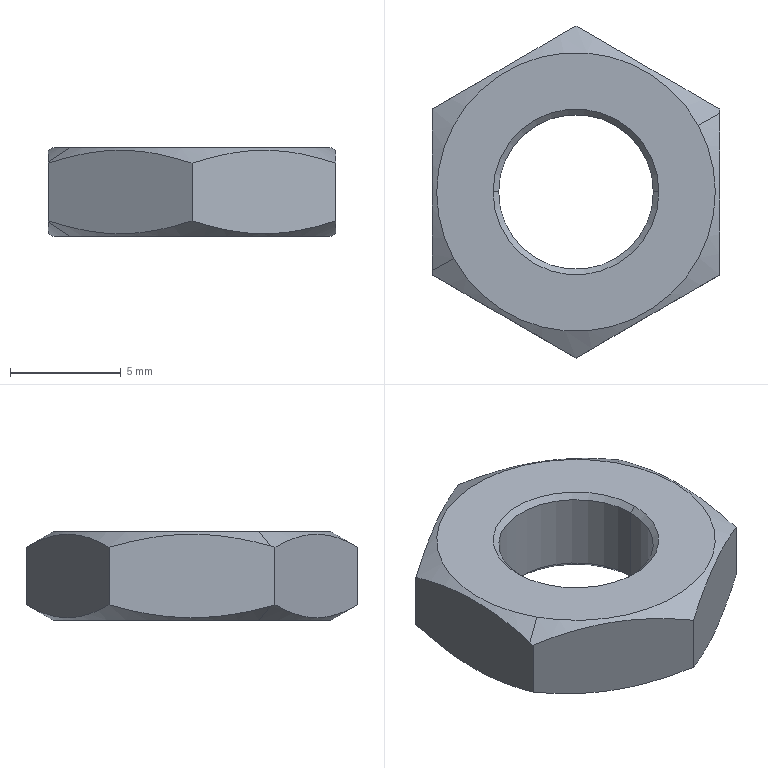Part | NX | features BREP 1 | 1 solid | 18 faces | box 13 x 15.011 x 4 mm | volume 421.241 mm3 | cone 8 | plane 8 | cylinder 2 | commonest cylinder face diameters 7 x2
STEP:
#1=CARTESIAN_POINT('',(3.75,0.,0.));
#2=VERTEX_POINT('',#1);
#3=CARTESIAN_POINT('',(3.5,0.,0.25));
#4=VERTEX_POINT('',#3);
#5=CARTESIAN_POINT('',(3.625,0.,0.125));
#6=DIRECTION('',(0.7071,0.,-0.7071));
#7=VECTOR('',#6,1000.);
#8=LINE('',#5,#7);
#9=EDGE_CURVE('',#2,#4,#8,.F.);
#10=ORIENTED_EDGE('',*,*,#9,.T.);
#11=CARTESIAN_POINT('',(-3.5,0.,0.25));
#12=VERTEX_POINT('',#11);
#13=CARTESIAN_POINT('',(0.,0.,0.25));
#14=DIRECTION('',(0.,0.,1.));
#15=DIRECTION('',(1.,0.,0.));
#16=AXIS2_PLACEMENT_3D('',#13,#14,#15);
#17=CIRCLE('',#16,3.5);
#18=EDGE_CURVE('',#4,#12,#17,.T.);
#19=ORIENTED_EDGE('',*,*,#18,.T.);
#20=CARTESIAN_POINT('',(-3.75,0.000000268,0.));
#21=VERTEX_POINT('',#20);
#22=CARTESIAN_POINT('',(-3.625,0.,0.125));
#23=DIRECTION('',(-0.7071,0.,-0.7071));
#24=VECTOR('',#23,1000.);
#25=LINE('',#22,#24);
#26=EDGE_CURVE('',#21,#12,#25,.F.);
#27=ORIENTED_EDGE('',*,*,#26,.F.);
#28=CARTESIAN_POINT('',(0.,0.,0.));
#29=DIRECTION('',(0.,0.,1.));
#30=DIRECTION('',(1.,0.,0.));
#31=AXIS2_PLACEMENT_3D('',#28,#29,#30);
#32=CIRCLE('',#31,3.75);
#33=EDGE_CURVE('',#2,#21,#32,.T.);
#34=ORIENTED_EDGE('',*,*,#33,.F.);
#35=EDGE_LOOP('',(#10,#19,#27,#34));
#36=FACE_BOUND('',#35,.T.);
#37=CARTESIAN_POINT('',(0.,0.,3.75));
#38=DIRECTION('',(0.,0.,-1.));
#39=DIRECTION('',(1.,0.,0.));
#40=AXIS2_PLACEMENT_3D('',#37,#38,#39);
#41=CONICAL_SURFACE('',#40,0.,0.7854);
#42=ADVANCED_FACE('',(#36),#41,.F.);
#43=ORIENTED_EDGE('',*,*,#26,.T.);
#44=CARTESIAN_POINT('',(0.,0.,0.25));
#45=DIRECTION('',(0.,0.,1.));
#46=DIRECTION('',(1.,0.,0.));
#47=AXIS2_PLACEMENT_3D('',#44,#45,#46);
#48=CIRCLE('',#47,3.5);
#49=EDGE_CURVE('',#12,#4,#48,.T.);
#50=ORIENTED_EDGE('',*,*,#49,.T.);
#51=ORIENTED_EDGE('',*,*,#9,.F.);
#52=CARTESIAN_POINT('',(0.,0.,0.));
#53=DIRECTION('',(0.,0.,1.));
#54=DIRECTION('',(1.,0.,0.));
#55=AXIS2_PLACEMENT_3D('',#52,#53,#54);
#56=CIRCLE('',#55,3.75);
#57=EDGE_CURVE('',#21,#2,#56,.T.);
#58=ORIENTED_EDGE('',*,*,#57,.F.);
#59=EDGE_LOOP('',(#43,#50,#51,#58));
#60=FACE_BOUND('',#59,.T.);
#61=CARTESIAN_POINT('',(0.,0.,3.75));
#62=DIRECTION('',(0.,0.,-1.));
#63=DIRECTION('',(-0.9924,0.1227,0.));
#64=AXIS2_PLACEMENT_3D('',#61,#62,#63);
#65=CONICAL_SURFACE('',#64,0.,0.7854);
#66=ADVANCED_FACE('',(#60),#65,.F.);
#67=ORIENTED_EDGE('',*,*,#49,.F.);
#68=CARTESIAN_POINT('',(-3.5,0.,3.75));
#69=VERTEX_POINT('',#68);
#70=CARTESIAN_POINT('',(-3.5,0.,2.));
#71=DIRECTION('',(0.,0.,1.));
#72=VECTOR('',#71,1000.);
#73=LINE('',#70,#72);
#74=EDGE_CURVE('',#12,#69,#73,.T.);
#75=ORIENTED_EDGE('',*,*,#74,.T.);
#76=CARTESIAN_POINT('',(3.5,0.,3.75));
#77=VERTEX_POINT('',#76);
#78=CARTESIAN_POINT('',(0.,0.,3.75));
#79=DIRECTION('',(0.,0.,1.));
#80=DIRECTION('',(1.,0.,0.));
#81=AXIS2_PLACEMENT_3D('',#78,#79,#80);
#82=CIRCLE('',#81,3.5);
#83=EDGE_CURVE('',#69,#77,#82,.T.);
#84=ORIENTED_EDGE('',*,*,#83,.T.);
#85=CARTESIAN_POINT('',(3.5,0.,2.));
#86=DIRECTION('',(0.,0.,1.));
#87=VECTOR('',#86,1000.);
#88=LINE('',#85,#87);
#89=EDGE_CURVE('',#4,#77,#88,.T.);
#90=ORIENTED_EDGE('',*,*,#89,.F.);
#91=EDGE_LOOP('',(#67,#75,#84,#90));
#92=FACE_BOUND('',#91,.T.);
#93=CARTESIAN_POINT('',(0.,0.,2.));
#94=DIRECTION('',(0.,0.,1.));
#95=DIRECTION('',(1.,0.,0.));
#96=AXIS2_PLACEMENT_3D('',#93,#94,#95);
#97=CYLINDRICAL_SURFACE('',#96,3.5);
#98=ADVANCED_FACE('',(#92),#97,.F.);
#99=ORIENTED_EDGE('',*,*,#18,.F.);
#100=ORIENTED_EDGE('',*,*,#89,.T.);
#101=CARTESIAN_POINT('',(0.,0.,3.75));
#102=DIRECTION('',(0.,0.,1.));
#103=DIRECTION('',(1.,0.,0.));
#104=AXIS2_PLACEMENT_3D('',#101,#102,#103);
#105=CIRCLE('',#104,3.5);
#106=EDGE_CURVE('',#77,#69,#105,.T.);
#107=ORIENTED_EDGE('',*,*,#106,.T.);
#108=ORIENTED_EDGE('',*,*,#74,.F.);
#109=EDGE_LOOP('',(#99,#100,#107,#108));
#110=FACE_BOUND('',#109,.T.);
#111=CARTESIAN_POINT('',(0.,0.,2.));
#112=DIRECTION('',(0.,0.,1.));
#113=DIRECTION('',(1.,0.,0.));
#114=AXIS2_PLACEMENT_3D('',#111,#112,#113);
#115=CYLINDRICAL_SURFACE('',#114,3.5);
#116=ADVANCED_FACE('',(#110),#115,.F.);
#117=ORIENTED_EDGE('',*,*,#57,.T.);
#118=ORIENTED_EDGE('',*,*,#33,.T.);
#119=EDGE_LOOP('',(#117,#118));
#120=FACE_BOUND('',#119,.T.);
#121=CARTESIAN_POINT('',(-5.529,-3.02,0.));
#122=VERTEX_POINT('',#121);
#123=CARTESIAN_POINT('',(5.529,3.02,0.));
#124=VERTEX_POINT('',#123);
#125=CARTESIAN_POINT('',(0.,0.,0.));
#126=DIRECTION('',(0.,0.,1.));
#127=DIRECTION('',(1.,0.,0.));
#128=AXIS2_PLACEMENT_3D('',#125,#126,#127);
#129=CIRCLE('',#128,6.3);
#130=EDGE_CURVE('',#122,#124,#129,.T.);
#131=ORIENTED_EDGE('',*,*,#130,.F.);
#132=CARTESIAN_POINT('',(0.,0.,0.));
#133=DIRECTION('',(0.,0.,1.));
#134=DIRECTION('',(1.,0.,0.));
#135=AXIS2_PLACEMENT_3D('',#132,#133,#134);
#136=CIRCLE('',#135,6.3);
#137=EDGE_CURVE('',#124,#122,#136,.T.);
#138=ORIENTED_EDGE('',*,*,#137,.F.);
#139=EDGE_LOOP('',(#131,#138));
#140=FACE_BOUND('',#139,.T.);
#141=CARTESIAN_POINT('',(0.,0.,0.));
#142=DIRECTION('',(0.,0.,1.));
#143=DIRECTION('',(1.,0.,0.));
#144=AXIS2_PLACEMENT_3D('',#141,#142,#143);
#145=PLANE('',#144);
#146=ADVANCED_FACE('',(#120,#140),#145,.F.);
#147=CARTESIAN_POINT('',(3.75,0.,4.));
#148=VERTEX_POINT('',#147);
#149=CARTESIAN_POINT('',(3.625,0.,3.875));
#150=DIRECTION('',(0.7071,0.,0.7071));
#151=VECTOR('',#150,1000.);
#152=LINE('',#149,#151);
#153=EDGE_CURVE('',#148,#77,#152,.F.);
#154=ORIENTED_EDGE('',*,*,#153,.F.);
#155=CARTESIAN_POINT('',(-3.75,0.000000268,4.));
#156=VERTEX_POINT('',#155);
#157=CARTESIAN_POINT('',(0.,0.,4.));
#158=DIRECTION('',(0.,0.,1.));
#159=DIRECTION('',(1.,0.,0.));
#160=AXIS2_PLACEMENT_3D('',#157,#158,#159);
#161=CIRCLE('',#160,3.75);
#162=EDGE_CURVE('',#148,#156,#161,.T.);
#163=ORIENTED_EDGE('',*,*,#162,.T.);
#164=CARTESIAN_POINT('',(-3.625,0.000000218,3.875));
#165=DIRECTION('',(-0.7071,0.000000043,0.7071));
#166=VECTOR('',#165,1000.);
#167=LINE('',#164,#166);
#168=EDGE_CURVE('',#156,#69,#167,.F.);
#169=ORIENTED_EDGE('',*,*,#168,.T.);
#170=ORIENTED_EDGE('',*,*,#106,.F.);
#171=EDGE_LOOP('',(#154,#163,#169,#170));
#172=FACE_BOUND('',#171,.T.);
#173=CARTESIAN_POINT('',(0.,0.,0.25));
#174=DIRECTION('',(0.,0.,1.));
#175=DIRECTION('',(1.,0.,0.));
#176=AXIS2_PLACEMENT_3D('',#173,#174,#175);
#177=CONICAL_SURFACE('',#176,0.,0.7854);
#178=ADVANCED_FACE('',(#172),#177,.F.);
#179=ORIENTED_EDGE('',*,*,#168,.F.);
#180=CARTESIAN_POINT('',(0.,0.,4.));
#181=DIRECTION('',(0.,0.,1.));
#182=DIRECTION('',(1.,0.,0.));
#183=AXIS2_PLACEMENT_3D('',#180,#181,#182);
#184=CIRCLE('',#183,3.75);
#185=EDGE_CURVE('',#156,#148,#184,.T.);
#186=ORIENTED_EDGE('',*,*,#185,.T.);
#187=ORIENTED_EDGE('',*,*,#153,.T.);
#188=ORIENTED_EDGE('',*,*,#83,.F.);
#189=EDGE_LOOP('',(#179,#186,#187,#188));
#190=FACE_BOUND('',#189,.T.);
#191=CARTESIAN_POINT('',(0.,0.,0.25));
#192=DIRECTION('',(0.,0.,1.));
#193=DIRECTION('',(-0.9924,0.1227,0.));
#194=AXIS2_PLACEMENT_3D('',#191,#192,#193);
#195=CONICAL_SURFACE('',#194,0.,0.7854);
#196=ADVANCED_FACE('',(#190),#195,.F.);
#197=ORIENTED_EDGE('',*,*,#162,.F.);
#198=ORIENTED_EDGE('',*,*,#185,.F.);
#199=EDGE_LOOP('',(#197,#198));
#200=FACE_BOUND('',#199,.T.);
#201=CARTESIAN_POINT('',(-5.529,-3.02,4.));
#202=VERTEX_POINT('',#201);
#203=CARTESIAN_POINT('',(5.529,3.02,4.));
#204=VERTEX_POINT('',#203);
#205=CARTESIAN_POINT('',(0.,0.,4.));
#206=DIRECTION('',(0.,0.,-1.));
#207=DIRECTION('',(-1.,0.,0.));
#208=AXIS2_PLACEMENT_3D('',#205,#206,#207);
#209=CIRCLE('',#208,6.3);
#210=EDGE_CURVE('',#202,#204,#209,.T.);
#211=ORIENTED_EDGE('',*,*,#210,.F.);
#212=CARTESIAN_POINT('',(0.,0.,4.));
#213=DIRECTION('',(0.,0.,-1.));
#214=DIRECTION('',(-1.,0.,0.));
#215=AXIS2_PLACEMENT_3D('',#212,#213,#214);
#216=CIRCLE('',#215,6.3);
#217=EDGE_CURVE('',#204,#202,#216,.T.);
#218=ORIENTED_EDGE('',*,*,#217,.F.);
#219=EDGE_LOOP('',(#211,#218));
#220=FACE_BOUND('',#219,.T.);
#221=CARTESIAN_POINT('',(0.,0.,4.));
#222=DIRECTION('',(0.,0.,1.));
#223=DIRECTION('',(1.,0.,0.));
#224=AXIS2_PLACEMENT_3D('',#221,#222,#223);
#225=PLANE('',#224);
#226=ADVANCED_FACE('',(#200,#220),#225,.T.);
#227=CARTESIAN_POINT('',(-6.5,-3.551,0.639));
#228=VERTEX_POINT('',#227);
#229=CARTESIAN_POINT('',(-6.788,-3.708,0.8285));
#230=DIRECTION('',(-0.76,-0.4152,0.5));
#231=VECTOR('',#230,1000.);
#232=LINE('',#229,#231);
#233=EDGE_CURVE('',#122,#228,#232,.T.);
#234=ORIENTED_EDGE('',*,*,#233,.F.);
#235=ORIENTED_EDGE('',*,*,#130,.T.);
#236=CARTESIAN_POINT('',(6.5,3.551,0.639));
#237=VERTEX_POINT('',#236);
#238=CARTESIAN_POINT('',(6.788,3.708,0.8285));
#239=DIRECTION('',(0.76,0.4152,0.5));
#240=VECTOR('',#239,1000.);
#241=LINE('',#238,#240);
#242=EDGE_CURVE('',#124,#237,#241,.T.);
#243=ORIENTED_EDGE('',*,*,#242,.T.);
#244=CARTESIAN_POINT('',(6.5,-3.753,0.696));
#245=VERTEX_POINT('',#244);
#246=CARTESIAN_POINT('',(6.5,3.551,0.639));
#247=CARTESIAN_POINT('',(6.5,3.11,0.517));
#248=CARTESIAN_POINT('',(6.5,2.701,0.4182));
#249=CARTESIAN_POINT('',(6.5,2.313,0.338));
#250=CARTESIAN_POINT('',(6.5,1.299,0.1635));
#251=CARTESIAN_POINT('',(6.5,0.3692,0.09904));
#252=CARTESIAN_POINT('',(6.5,-0.2087,0.09497));
#253=CARTESIAN_POINT('',(6.5,-1.197,0.1497));
#254=CARTESIAN_POINT('',(6.5,-2.27,0.3265));
#255=CARTESIAN_POINT('',(6.5,-2.727,0.4207));
#256=CARTESIAN_POINT('',(6.5,-3.216,0.5412));
#257=CARTESIAN_POINT('',(6.5,-3.753,0.696));
#258=B_SPLINE_CURVE_WITH_KNOTS('',5,(#246,#247,#248,#249,#250,#251,#252,#253,#254,#255,#256,#257),.UNSPECIFIED.,.F.,.F.,(6,3,3,6),(0.,26.231,71.597,102.705),.UNSPECIFIED.);
#259=EDGE_CURVE('',#237,#245,#258,.T.);
#260=ORIENTED_EDGE('',*,*,#259,.T.);
#261=CARTESIAN_POINT('',(0.,-7.506,0.696));
#262=VERTEX_POINT('',#261);
#263=CARTESIAN_POINT('',(0.,-7.506,0.696));
#264=CARTESIAN_POINT('',(0.3698,-7.292,0.5728));
#265=CARTESIAN_POINT('',(0.7137,-7.094,0.4713));
#266=CARTESIAN_POINT('',(1.039,-6.906,0.3874));
#267=CARTESIAN_POINT('',(2.057,-6.318,0.1629));
#268=CARTESIAN_POINT('',(2.963,-5.795,0.08633));
#269=CARTESIAN_POINT('',(3.578,-5.44,0.08782));
#270=CARTESIAN_POINT('',(4.478,-4.92,0.1681));
#271=CARTESIAN_POINT('',(5.491,-4.335,0.3951));
#272=CARTESIAN_POINT('',(5.807,-4.153,0.4774));
#273=CARTESIAN_POINT('',(6.141,-3.96,0.5765));
#274=CARTESIAN_POINT('',(6.5,-3.753,0.696));
#275=B_SPLINE_CURVE_WITH_KNOTS('',5,(#263,#264,#265,#266,#267,#268,#269,#270,#271,#272,#273,#274),.UNSPECIFIED.,.F.,.F.,(6,3,3,6),(0.,24.765,81.109,105.126),.UNSPECIFIED.);
#276=EDGE_CURVE('',#262,#245,#275,.T.);
#277=ORIENTED_EDGE('',*,*,#276,.F.);
#278=CARTESIAN_POINT('',(-6.5,-3.753,0.696));
#279=VERTEX_POINT('',#278);
#280=CARTESIAN_POINT('',(-6.5,-3.753,0.696));
#281=CARTESIAN_POINT('',(-6.13,-3.966,0.5728));
#282=CARTESIAN_POINT('',(-5.786,-4.165,0.4713));
#283=CARTESIAN_POINT('',(-5.461,-4.352,0.3874));
#284=CARTESIAN_POINT('',(-4.443,-4.94,0.1629));
#285=CARTESIAN_POINT('',(-3.537,-5.464,0.08633));
#286=CARTESIAN_POINT('',(-2.922,-5.819,0.08782));
#287=CARTESIAN_POINT('',(-2.022,-6.338,0.1681));
#288=CARTESIAN_POINT('',(-1.009,-6.923,0.3951));
#289=CARTESIAN_POINT('',(-0.6929,-7.106,0.4774));
#290=CARTESIAN_POINT('',(-0.3586,-7.299,0.5765));
#291=CARTESIAN_POINT('',(0.,-7.506,0.696));
#292=B_SPLINE_CURVE_WITH_KNOTS('',5,(#280,#281,#282,#283,#284,#285,#286,#287,#288,#289,#290,#291),.UNSPECIFIED.,.F.,.F.,(6,3,3,6),(0.,24.765,81.109,105.126),.UNSPECIFIED.);
#293=EDGE_CURVE('',#279,#262,#292,.T.);
#294=ORIENTED_EDGE('',*,*,#293,.F.);
#295=CARTESIAN_POINT('',(-6.5,-3.551,0.639));
#296=CARTESIAN_POINT('',(-6.5,-3.591,0.65));
#297=CARTESIAN_POINT('',(-6.5,-3.631,0.6612));
#298=CARTESIAN_POINT('',(-6.5,-3.671,0.6726));
#299=CARTESIAN_POINT('',(-6.5,-3.712,0.6842));
#300=CARTESIAN_POINT('',(-6.5,-3.753,0.696));
#301=B_SPLINE_CURVE_WITH_KNOTS('',5,(#295,#296,#297,#298,#299,#300),.UNSPECIFIED.,.F.,.F.,(6,6),(0.,2.372),.UNSPECIFIED.);
#302=EDGE_CURVE('',#228,#279,#301,.T.);
#303=ORIENTED_EDGE('',*,*,#302,.F.);
#304=EDGE_LOOP('',(#234,#235,#243,#260,#277,#294,#303));
#305=FACE_BOUND('',#304,.T.);
#306=CARTESIAN_POINT('',(0.,0.,0.));
#307=DIRECTION('',(0.,0.,1.));
#308=DIRECTION('',(-0.8776,-0.4794,0.));
#309=AXIS2_PLACEMENT_3D('',#306,#307,#308);
#310=CONICAL_SURFACE('',#309,6.3,1.047);
#311=ADVANCED_FACE('',(#305),#310,.T.);
#312=ORIENTED_EDGE('',*,*,#242,.F.);
#313=ORIENTED_EDGE('',*,*,#137,.T.);
#314=ORIENTED_EDGE('',*,*,#233,.T.);
#315=CARTESIAN_POINT('',(-6.5,3.753,0.696));
#316=VERTEX_POINT('',#315);
#317=CARTESIAN_POINT('',(-6.5,-3.551,0.639));
#318=CARTESIAN_POINT('',(-6.5,-3.11,0.517));
#319=CARTESIAN_POINT('',(-6.5,-2.701,0.4182));
#320=CARTESIAN_POINT('',(-6.5,-2.313,0.338));
#321=CARTESIAN_POINT('',(-6.5,-1.299,0.1635));
#322=CARTESIAN_POINT('',(-6.5,-0.3692,0.09904));
#323=CARTESIAN_POINT('',(-6.5,0.2087,0.09497));
#324=CARTESIAN_POINT('',(-6.5,1.197,0.1497));
#325=CARTESIAN_POINT('',(-6.5,2.27,0.3265));
#326=CARTESIAN_POINT('',(-6.5,2.727,0.4207));
#327=CARTESIAN_POINT('',(-6.5,3.216,0.5412));
#328=CARTESIAN_POINT('',(-6.5,3.753,0.696));
#329=B_SPLINE_CURVE_WITH_KNOTS('',5,(#317,#318,#319,#320,#321,#322,#323,#324,#325,#326,#327,#328),.UNSPECIFIED.,.F.,.F.,(6,3,3,6),(0.,26.231,71.597,102.705),.UNSPECIFIED.);
#330=EDGE_CURVE('',#228,#316,#329,.T.);
#331=ORIENTED_EDGE('',*,*,#330,.T.);
#332=CARTESIAN_POINT('',(0.,7.506,0.696));
#333=VERTEX_POINT('',#332);
#334=CARTESIAN_POINT('',(0.,7.506,0.696));
#335=CARTESIAN_POINT('',(-0.3698,7.292,0.5728));
#336=CARTESIAN_POINT('',(-0.7137,7.094,0.4713));
#337=CARTESIAN_POINT('',(-1.039,6.906,0.3874));
#338=CARTESIAN_POINT('',(-2.057,6.318,0.1629));
#339=CARTESIAN_POINT('',(-2.963,5.795,0.08633));
#340=CARTESIAN_POINT('',(-3.578,5.44,0.08782));
#341=CARTESIAN_POINT('',(-4.478,4.92,0.1681));
#342=CARTESIAN_POINT('',(-5.491,4.335,0.3951));
#343=CARTESIAN_POINT('',(-5.807,4.153,0.4774));
#344=CARTESIAN_POINT('',(-6.141,3.96,0.5765));
#345=CARTESIAN_POINT('',(-6.5,3.753,0.696));
#346=B_SPLINE_CURVE_WITH_KNOTS('',5,(#334,#335,#336,#337,#338,#339,#340,#341,#342,#343,#344,#345),.UNSPECIFIED.,.F.,.F.,(6,3,3,6),(0.,24.765,81.109,105.126),.UNSPECIFIED.);
#347=EDGE_CURVE('',#333,#316,#346,.T.);
#348=ORIENTED_EDGE('',*,*,#347,.F.);
#349=CARTESIAN_POINT('',(6.5,3.753,0.696));
#350=VERTEX_POINT('',#349);
#351=CARTESIAN_POINT('',(6.5,3.753,0.696));
#352=CARTESIAN_POINT('',(6.13,3.966,0.5728));
#353=CARTESIAN_POINT('',(5.786,4.165,0.4713));
#354=CARTESIAN_POINT('',(5.461,4.352,0.3874));
#355=CARTESIAN_POINT('',(4.443,4.94,0.1629));
#356=CARTESIAN_POINT('',(3.537,5.464,0.08633));
#357=CARTESIAN_POINT('',(2.922,5.819,0.08782));
#358=CARTESIAN_POINT('',(2.022,6.338,0.1681));
#359=CARTESIAN_POINT('',(1.009,6.923,0.3951));
#360=CARTESIAN_POINT('',(0.6929,7.106,0.4774));
#361=CARTESIAN_POINT('',(0.3586,7.299,0.5765));
#362=CARTESIAN_POINT('',(0.,7.506,0.696));
#363=B_SPLINE_CURVE_WITH_KNOTS('',5,(#351,#352,#353,#354,#355,#356,#357,#358,#359,#360,#361,#362),.UNSPECIFIED.,.F.,.F.,(6,3,3,6),(0.,24.765,81.109,105.126),.UNSPECIFIED.);
#364=EDGE_CURVE('',#350,#333,#363,.T.);
#365=ORIENTED_EDGE('',*,*,#364,.F.);
#366=CARTESIAN_POINT('',(6.5,3.551,0.639));
#367=CARTESIAN_POINT('',(6.5,3.591,0.65));
#368=CARTESIAN_POINT('',(6.5,3.631,0.6612));
#369=CARTESIAN_POINT('',(6.5,3.671,0.6726));
#370=CARTESIAN_POINT('',(6.5,3.712,0.6842));
#371=CARTESIAN_POINT('',(6.5,3.753,0.696));
#372=B_SPLINE_CURVE_WITH_KNOTS('',5,(#366,#367,#368,#369,#370,#371),.UNSPECIFIED.,.F.,.F.,(6,6),(0.,2.372),.UNSPECIFIED.);
#373=EDGE_CURVE('',#237,#350,#372,.T.);
#374=ORIENTED_EDGE('',*,*,#373,.F.);
#375=EDGE_LOOP('',(#312,#313,#314,#331,#348,#365,#374));
#376=FACE_BOUND('',#375,.T.);
#377=CARTESIAN_POINT('',(0.,0.,0.));
#378=DIRECTION('',(0.,0.,1.));
#379=DIRECTION('',(-0.8776,-0.4794,0.));
#380=AXIS2_PLACEMENT_3D('',#377,#378,#379);
#381=CONICAL_SURFACE('',#380,6.3,1.047);
#382=ADVANCED_FACE('',(#376),#381,.T.);
#383=CARTESIAN_POINT('',(6.5,-3.753,3.304));
#384=VERTEX_POINT('',#383);
#385=CARTESIAN_POINT('',(6.5,-3.753,2.));
#386=DIRECTION('',(0.,0.,1.));
#387=VECTOR('',#386,1000.);
#388=LINE('',#385,#387);
#389=EDGE_CURVE('',#245,#384,#388,.T.);
#390=ORIENTED_EDGE('',*,*,#389,.T.);
#391=CARTESIAN_POINT('',(0.,-7.506,3.304));
#392=VERTEX_POINT('',#391);
#393=CARTESIAN_POINT('',(0.,-7.506,3.304));
#394=CARTESIAN_POINT('',(0.4257,-7.26,3.446));
#395=CARTESIAN_POINT('',(0.8172,-7.034,3.559));
#396=CARTESIAN_POINT('',(1.185,-6.822,3.649));
#397=CARTESIAN_POINT('',(2.094,-6.297,3.834));
#398=CARTESIAN_POINT('',(2.925,-5.817,3.901));
#399=CARTESIAN_POINT('',(3.425,-5.528,3.905));
#400=CARTESIAN_POINT('',(4.282,-5.033,3.851));
#401=CARTESIAN_POINT('',(5.212,-4.497,3.674));
#402=CARTESIAN_POINT('',(5.609,-4.267,3.58));
#403=CARTESIAN_POINT('',(6.034,-4.022,3.459));
#404=CARTESIAN_POINT('',(6.5,-3.753,3.304));
#405=B_SPLINE_CURVE_WITH_KNOTS('',5,(#393,#394,#395,#396,#397,#398,#399,#400,#401,#402,#403,#404),.UNSPECIFIED.,.F.,.F.,(6,3,3,6),(0.,28.513,73.873,105.079),.UNSPECIFIED.);
#406=EDGE_CURVE('',#392,#384,#405,.T.);
#407=ORIENTED_EDGE('',*,*,#406,.F.);
#408=CARTESIAN_POINT('',(0.,-7.506,2.));
#409=DIRECTION('',(0.,0.,1.));
#410=VECTOR('',#409,1000.);
#411=LINE('',#408,#410);
#412=EDGE_CURVE('',#262,#392,#411,.T.);
#413=ORIENTED_EDGE('',*,*,#412,.F.);
#414=ORIENTED_EDGE('',*,*,#276,.T.);
#415=EDGE_LOOP('',(#390,#407,#413,#414));
#416=FACE_BOUND('',#415,.T.);
#417=CARTESIAN_POINT('',(0.,-7.506,0.));
#418=DIRECTION('',(0.5,-0.866,0.));
#419=DIRECTION('',(0.866,0.5,0.));
#420=AXIS2_PLACEMENT_3D('',#417,#418,#419);
#421=PLANE('',#420);
#422=ADVANCED_FACE('',(#416),#421,.T.);
#423=ORIENTED_EDGE('',*,*,#412,.T.);
#424=CARTESIAN_POINT('',(-6.5,-3.753,3.304));
#425=VERTEX_POINT('',#424);
#426=CARTESIAN_POINT('',(-6.5,-3.753,3.304));
#427=CARTESIAN_POINT('',(-6.074,-3.999,3.446));
#428=CARTESIAN_POINT('',(-5.683,-4.225,3.559));
#429=CARTESIAN_POINT('',(-5.315,-4.437,3.649));
#430=CARTESIAN_POINT('',(-4.406,-4.962,3.834));
#431=CARTESIAN_POINT('',(-3.575,-5.441,3.901));
#432=CARTESIAN_POINT('',(-3.075,-5.73,3.905));
#433=CARTESIAN_POINT('',(-2.218,-6.225,3.851));
#434=CARTESIAN_POINT('',(-1.288,-6.762,3.674));
#435=CARTESIAN_POINT('',(-0.8908,-6.991,3.58));
#436=CARTESIAN_POINT('',(-0.466,-7.237,3.459));
#437=CARTESIAN_POINT('',(0.,-7.506,3.304));
#438=B_SPLINE_CURVE_WITH_KNOTS('',5,(#426,#427,#428,#429,#430,#431,#432,#433,#434,#435,#436,#437),.UNSPECIFIED.,.F.,.F.,(6,3,3,6),(0.,28.513,73.873,105.079),.UNSPECIFIED.);
#439=EDGE_CURVE('',#425,#392,#438,.T.);
#440=ORIENTED_EDGE('',*,*,#439,.F.);
#441=CARTESIAN_POINT('',(-6.5,-3.753,2.));
#442=DIRECTION('',(0.,0.,1.));
#443=VECTOR('',#442,1000.);
#444=LINE('',#441,#443);
#445=EDGE_CURVE('',#279,#425,#444,.T.);
#446=ORIENTED_EDGE('',*,*,#445,.F.);
#447=ORIENTED_EDGE('',*,*,#293,.T.);
#448=EDGE_LOOP('',(#423,#440,#446,#447));
#449=FACE_BOUND('',#448,.T.);
#450=CARTESIAN_POINT('',(-6.5,-3.753,0.));
#451=DIRECTION('',(-0.5,-0.866,0.));
#452=DIRECTION('',(0.866,-0.5,0.));
#453=AXIS2_PLACEMENT_3D('',#450,#451,#452);
#454=PLANE('',#453);
#455=ADVANCED_FACE('',(#449),#454,.T.);
#456=ORIENTED_EDGE('',*,*,#445,.T.);
#457=CARTESIAN_POINT('',(-6.5,-3.551,3.361));
#458=VERTEX_POINT('',#457);
#459=CARTESIAN_POINT('',(-6.5,-3.551,3.361));
#460=CARTESIAN_POINT('',(-6.5,-3.617,3.343));
#461=CARTESIAN_POINT('',(-6.5,-3.685,3.324));
#462=CARTESIAN_POINT('',(-6.5,-3.753,3.304));
#463=B_SPLINE_CURVE_WITH_KNOTS('',3,(#459,#460,#461,#462),.UNSPECIFIED.,.F.,.F.,(4,4),(0.,2.372),.UNSPECIFIED.);
#464=EDGE_CURVE('',#458,#425,#463,.T.);
#465=ORIENTED_EDGE('',*,*,#464,.F.);
#466=CARTESIAN_POINT('',(-6.5,3.753,3.304));
#467=VERTEX_POINT('',#466);
#468=CARTESIAN_POINT('',(-6.5,-3.551,3.361));
#469=CARTESIAN_POINT('',(-6.5,-2.869,3.55));
#470=CARTESIAN_POINT('',(-6.5,-1.568,3.822));
#471=CARTESIAN_POINT('',(-6.5,0.07587,3.92));
#472=CARTESIAN_POINT('',(-6.5,1.727,3.8));
#473=CARTESIAN_POINT('',(-6.5,3.055,3.505));
#474=CARTESIAN_POINT('',(-6.5,3.753,3.304));
#475=B_SPLINE_CURVE_WITH_KNOTS('',3,(#468,#469,#470,#471,#472,#473,#474),.UNSPECIFIED.,.F.,.F.,(4,1,1,1,4),(0.,0.25,0.5,0.75,1.),.UNSPECIFIED.);
#476=EDGE_CURVE('',#458,#467,#475,.T.);
#477=ORIENTED_EDGE('',*,*,#476,.T.);
#478=CARTESIAN_POINT('',(-6.5,3.753,2.));
#479=DIRECTION('',(0.,0.,1.));
#480=VECTOR('',#479,1000.);
#481=LINE('',#478,#480);
#482=EDGE_CURVE('',#316,#467,#481,.T.);
#483=ORIENTED_EDGE('',*,*,#482,.F.);
#484=ORIENTED_EDGE('',*,*,#330,.F.);
#485=ORIENTED_EDGE('',*,*,#302,.T.);
#486=EDGE_LOOP('',(#456,#465,#477,#483,#484,#485));
#487=FACE_BOUND('',#486,.T.);
#488=CARTESIAN_POINT('',(-6.5,3.753,0.));
#489=DIRECTION('',(-1.,0.,0.));
#490=DIRECTION('',(0.,-1.,0.));
#491=AXIS2_PLACEMENT_3D('',#488,#489,#490);
#492=PLANE('',#491);
#493=ADVANCED_FACE('',(#487),#492,.T.);
#494=ORIENTED_EDGE('',*,*,#482,.T.);
#495=CARTESIAN_POINT('',(0.,7.506,3.304));
#496=VERTEX_POINT('',#495);
#497=CARTESIAN_POINT('',(0.,7.506,3.304));
#498=CARTESIAN_POINT('',(-0.4257,7.26,3.446));
#499=CARTESIAN_POINT('',(-0.8172,7.034,3.559));
#500=CARTESIAN_POINT('',(-1.185,6.822,3.649));
#501=CARTESIAN_POINT('',(-2.094,6.297,3.834));
#502=CARTESIAN_POINT('',(-2.925,5.817,3.901));
#503=CARTESIAN_POINT('',(-3.425,5.528,3.905));
#504=CARTESIAN_POINT('',(-4.282,5.033,3.851));
#505=CARTESIAN_POINT('',(-5.212,4.497,3.674));
#506=CARTESIAN_POINT('',(-5.609,4.267,3.58));
#507=CARTESIAN_POINT('',(-6.034,4.022,3.459));
#508=CARTESIAN_POINT('',(-6.5,3.753,3.304));
#509=B_SPLINE_CURVE_WITH_KNOTS('',5,(#497,#498,#499,#500,#501,#502,#503,#504,#505,#506,#507,#508),.UNSPECIFIED.,.F.,.F.,(6,3,3,6),(0.,28.513,73.873,105.079),.UNSPECIFIED.);
#510=EDGE_CURVE('',#496,#467,#509,.T.);
#511=ORIENTED_EDGE('',*,*,#510,.F.);
#512=CARTESIAN_POINT('',(0.,7.506,2.));
#513=DIRECTION('',(0.,0.,1.));
#514=VECTOR('',#513,1000.);
#515=LINE('',#512,#514);
#516=EDGE_CURVE('',#333,#496,#515,.T.);
#517=ORIENTED_EDGE('',*,*,#516,.F.);
#518=ORIENTED_EDGE('',*,*,#347,.T.);
#519=EDGE_LOOP('',(#494,#511,#517,#518));
#520=FACE_BOUND('',#519,.T.);
#521=CARTESIAN_POINT('',(0.,7.506,0.));
#522=DIRECTION('',(-0.5,0.866,0.));
#523=DIRECTION('',(-0.866,-0.5,0.));
#524=AXIS2_PLACEMENT_3D('',#521,#522,#523);
#525=PLANE('',#524);
#526=ADVANCED_FACE('',(#520),#525,.T.);
#527=ORIENTED_EDGE('',*,*,#516,.T.);
#528=CARTESIAN_POINT('',(6.5,3.753,3.304));
#529=VERTEX_POINT('',#528);
#530=CARTESIAN_POINT('',(6.5,3.753,3.304));
#531=CARTESIAN_POINT('',(6.074,3.999,3.446));
#532=CARTESIAN_POINT('',(5.683,4.225,3.559));
#533=CARTESIAN_POINT('',(5.315,4.437,3.649));
#534=CARTESIAN_POINT('',(4.406,4.962,3.834));
#535=CARTESIAN_POINT('',(3.575,5.441,3.901));
#536=CARTESIAN_POINT('',(3.075,5.73,3.905));
#537=CARTESIAN_POINT('',(2.218,6.225,3.851));
#538=CARTESIAN_POINT('',(1.288,6.762,3.674));
#539=CARTESIAN_POINT('',(0.8908,6.991,3.58));
#540=CARTESIAN_POINT('',(0.466,7.237,3.459));
#541=CARTESIAN_POINT('',(0.,7.506,3.304));
#542=B_SPLINE_CURVE_WITH_KNOTS('',5,(#530,#531,#532,#533,#534,#535,#536,#537,#538,#539,#540,#541),.UNSPECIFIED.,.F.,.F.,(6,3,3,6),(0.,28.513,73.873,105.079),.UNSPECIFIED.);
#543=EDGE_CURVE('',#529,#496,#542,.T.);
#544=ORIENTED_EDGE('',*,*,#543,.F.);
#545=CARTESIAN_POINT('',(6.5,3.753,2.));
#546=DIRECTION('',(0.,0.,1.));
#547=VECTOR('',#546,1000.);
#548=LINE('',#545,#547);
#549=EDGE_CURVE('',#350,#529,#548,.T.);
#550=ORIENTED_EDGE('',*,*,#549,.F.);
#551=ORIENTED_EDGE('',*,*,#364,.T.);
#552=EDGE_LOOP('',(#527,#544,#550,#551));
#553=FACE_BOUND('',#552,.T.);
#554=CARTESIAN_POINT('',(6.5,3.753,0.));
#555=DIRECTION('',(0.5,0.866,0.));
#556=DIRECTION('',(-0.866,0.5,0.));
#557=AXIS2_PLACEMENT_3D('',#554,#555,#556);
#558=PLANE('',#557);
#559=ADVANCED_FACE('',(#553),#558,.T.);
#560=ORIENTED_EDGE('',*,*,#549,.T.);
#561=CARTESIAN_POINT('',(6.5,3.551,3.361));
#562=VERTEX_POINT('',#561);
#563=CARTESIAN_POINT('',(6.5,3.551,3.361));
#564=CARTESIAN_POINT('',(6.5,3.617,3.343));
#565=CARTESIAN_POINT('',(6.5,3.685,3.324));
#566=CARTESIAN_POINT('',(6.5,3.753,3.304));
#567=B_SPLINE_CURVE_WITH_KNOTS('',3,(#563,#564,#565,#566),.UNSPECIFIED.,.F.,.F.,(4,4),(0.,2.372),.UNSPECIFIED.);
#568=EDGE_CURVE('',#562,#529,#567,.T.);
#569=ORIENTED_EDGE('',*,*,#568,.F.);
#570=CARTESIAN_POINT('',(6.5,3.551,3.361));
#571=CARTESIAN_POINT('',(6.5,2.869,3.55));
#572=CARTESIAN_POINT('',(6.5,1.568,3.822));
#573=CARTESIAN_POINT('',(6.5,-0.07587,3.92));
#574=CARTESIAN_POINT('',(6.5,-1.727,3.8));
#575=CARTESIAN_POINT('',(6.5,-3.055,3.505));
#576=CARTESIAN_POINT('',(6.5,-3.753,3.304));
#577=B_SPLINE_CURVE_WITH_KNOTS('',3,(#570,#571,#572,#573,#574,#575,#576),.UNSPECIFIED.,.F.,.F.,(4,1,1,1,4),(0.,0.25,0.5,0.75,1.),.UNSPECIFIED.);
#578=EDGE_CURVE('',#562,#384,#577,.T.);
#579=ORIENTED_EDGE('',*,*,#578,.T.);
#580=ORIENTED_EDGE('',*,*,#389,.F.);
#581=ORIENTED_EDGE('',*,*,#259,.F.);
#582=ORIENTED_EDGE('',*,*,#373,.T.);
#583=EDGE_LOOP('',(#560,#569,#579,#580,#581,#582));
#584=FACE_BOUND('',#583,.T.);
#585=CARTESIAN_POINT('',(6.5,-3.753,0.));
#586=DIRECTION('',(1.,0.,0.));
#587=DIRECTION('',(0.,1.,0.));
#588=AXIS2_PLACEMENT_3D('',#585,#586,#587);
#589=PLANE('',#588);
#590=ADVANCED_FACE('',(#584),#589,.T.);
#591=CARTESIAN_POINT('',(8.684,4.744,1.924));
#592=DIRECTION('',(0.76,0.4152,-0.5));
#593=VECTOR('',#592,1000.);
#594=LINE('',#591,#593);
#595=EDGE_CURVE('',#562,#204,#594,.F.);
#596=ORIENTED_EDGE('',*,*,#595,.T.);
#597=ORIENTED_EDGE('',*,*,#217,.T.);
#598=CARTESIAN_POINT('',(-8.684,-4.744,1.924));
#599=DIRECTION('',(-0.76,-0.4152,-0.5));
#600=VECTOR('',#599,1000.);
#601=LINE('',#598,#600);
#602=EDGE_CURVE('',#458,#202,#601,.F.);
#603=ORIENTED_EDGE('',*,*,#602,.F.);
#604=ORIENTED_EDGE('',*,*,#464,.T.);
#605=ORIENTED_EDGE('',*,*,#439,.T.);
#606=ORIENTED_EDGE('',*,*,#406,.T.);
#607=ORIENTED_EDGE('',*,*,#578,.F.);
#608=EDGE_LOOP('',(#596,#597,#603,#604,#605,#606,#607));
#609=FACE_BOUND('',#608,.T.);
#610=CARTESIAN_POINT('',(0.,0.,4.));
#611=DIRECTION('',(0.,0.,-1.));
#612=DIRECTION('',(-0.8776,-0.4794,0.));
#613=AXIS2_PLACEMENT_3D('',#610,#611,#612);
#614=CONICAL_SURFACE('',#613,6.3,1.047);
#615=ADVANCED_FACE('',(#609),#614,.T.);
#616=ORIENTED_EDGE('',*,*,#602,.T.);
#617=ORIENTED_EDGE('',*,*,#210,.T.);
#618=ORIENTED_EDGE('',*,*,#595,.F.);
#619=ORIENTED_EDGE('',*,*,#568,.T.);
#620=ORIENTED_EDGE('',*,*,#543,.T.);
#621=ORIENTED_EDGE('',*,*,#510,.T.);
#622=ORIENTED_EDGE('',*,*,#476,.F.);
#623=EDGE_LOOP('',(#616,#617,#618,#619,#620,#621,#622));
#624=FACE_BOUND('',#623,.T.);
#625=CARTESIAN_POINT('',(0.,0.,4.));
#626=DIRECTION('',(0.,0.,-1.));
#627=DIRECTION('',(-0.8776,-0.4794,0.));
#628=AXIS2_PLACEMENT_3D('',#625,#626,#627);
#629=CONICAL_SURFACE('',#628,6.3,1.047);
#630=ADVANCED_FACE('',(#624),#629,.T.);
#631=CLOSED_SHELL('',(#42,#66,#98,#116,#146,#178,#196,#226,#311,#382,#422,#455,#493,#526,#559,#590,#615,#630));
#632=MANIFOLD_SOLID_BREP('',#631);
#633=(LENGTH_UNIT()NAMED_UNIT(*)SI_UNIT(.MILLI.,.METRE.));
#634=UNCERTAINTY_MEASURE_WITH_UNIT(LENGTH_MEASURE(0.0508),#633,'','');
#635=(NAMED_UNIT(*)PLANE_ANGLE_UNIT()SI_UNIT($,.RADIAN.));
#636=(NAMED_UNIT(*)SI_UNIT($,.STERADIAN.)SOLID_ANGLE_UNIT());
#637=(GEOMETRIC_REPRESENTATION_CONTEXT(3)GLOBAL_UNCERTAINTY_ASSIGNED_CONTEXT((#634))GLOBAL_UNIT_ASSIGNED_CONTEXT((#633,#635,#636))REPRESENTATION_CONTEXT('',''));
#638=ADVANCED_BREP_SHAPE_REPRESENTATION('',(#632),#637);